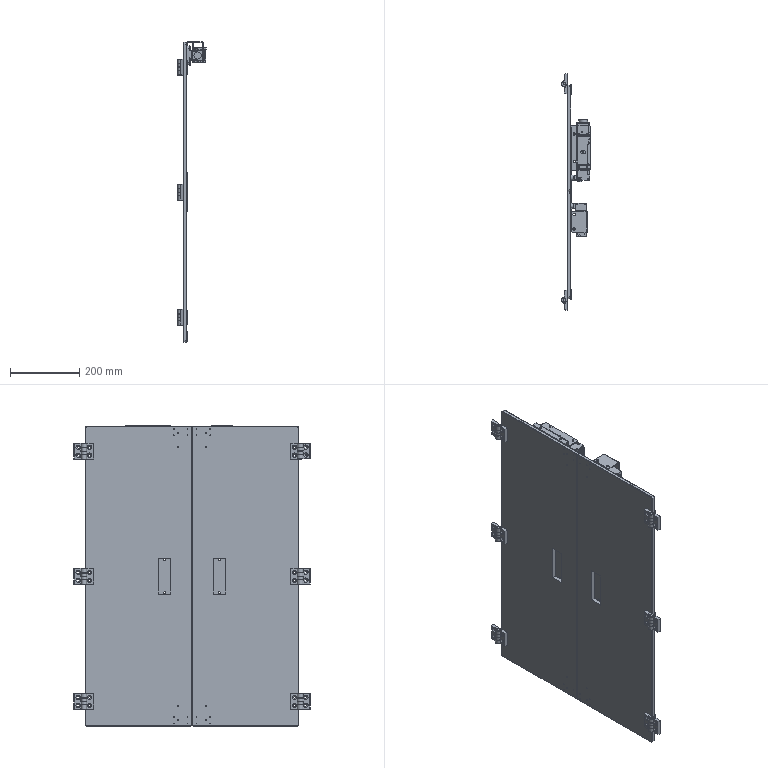Part | NX | 42 solids | 1479 faces | box 83.2 x 686 x 870.5 mm | volume 5815414 mm3 | plane 1082 | cylinder 341 | cone 53 | spline 2 | torus 1 | commonest cylinder face diameters 8 x39 6 x31 4 x30 7 x25 6.5 x24 16 x24